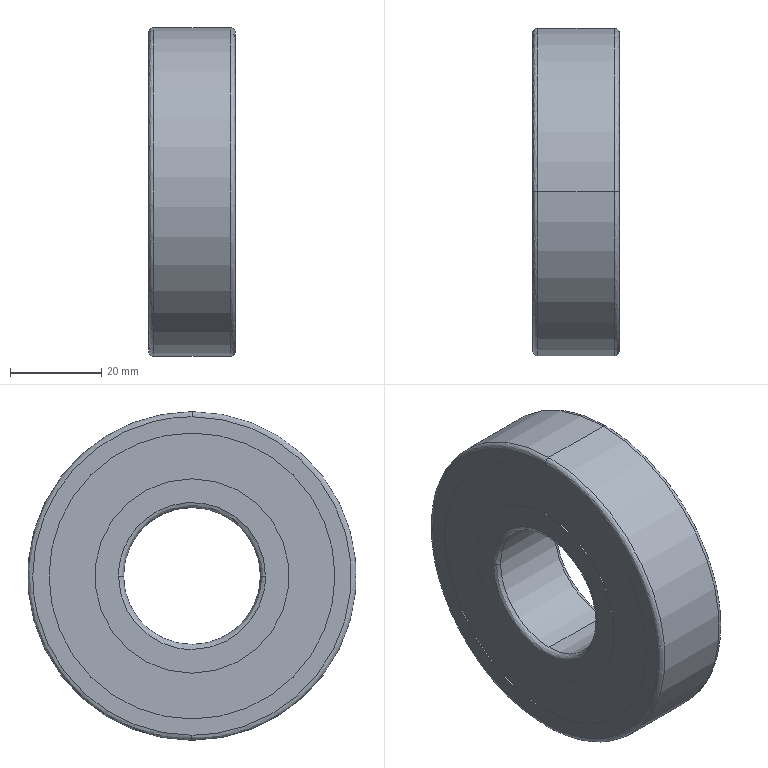Part | SolidWorks | features BaseBody 14 | 14 solids | 74 faces | box 19 x 72 x 72 mm | volume 45746 mm3 | spline 34 | cylinder 28 | plane 12 | commonest cylinder face diameters 42.6 x8 62.65 x8 44.7 x4 59.5 x4 30 x2 72 x2